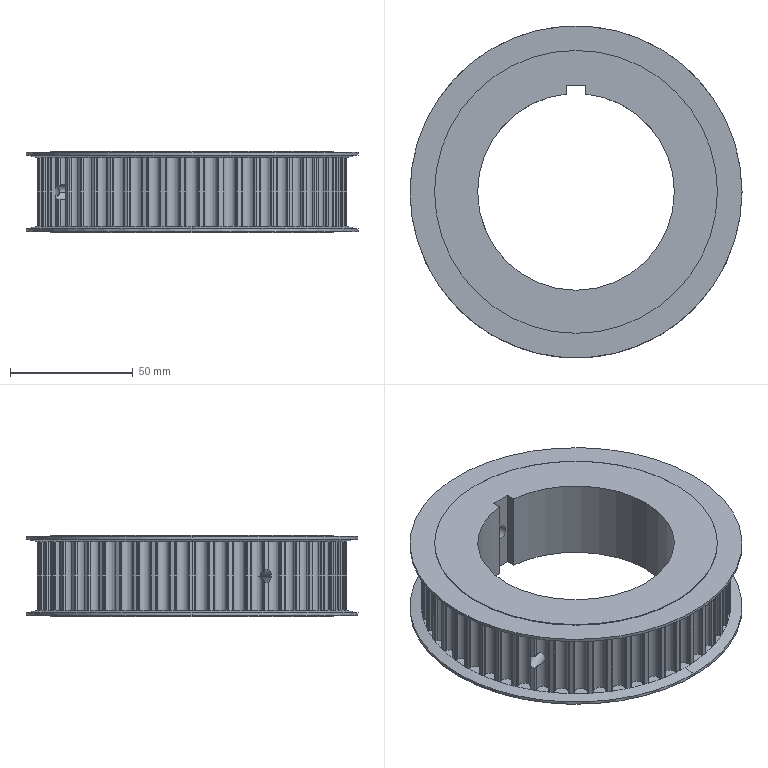Part | SolidWorks | features BaseBody 1 | 1 solid | 484 faces | box 135 x 135 x 33 mm | volume 226283 mm3 | cylinder 269 | plane 211 | cone 4 | commonest cylinder face diameters 0.81 x127 5.184 x75 125.95 x52 6 x4 115 x4 135 x4